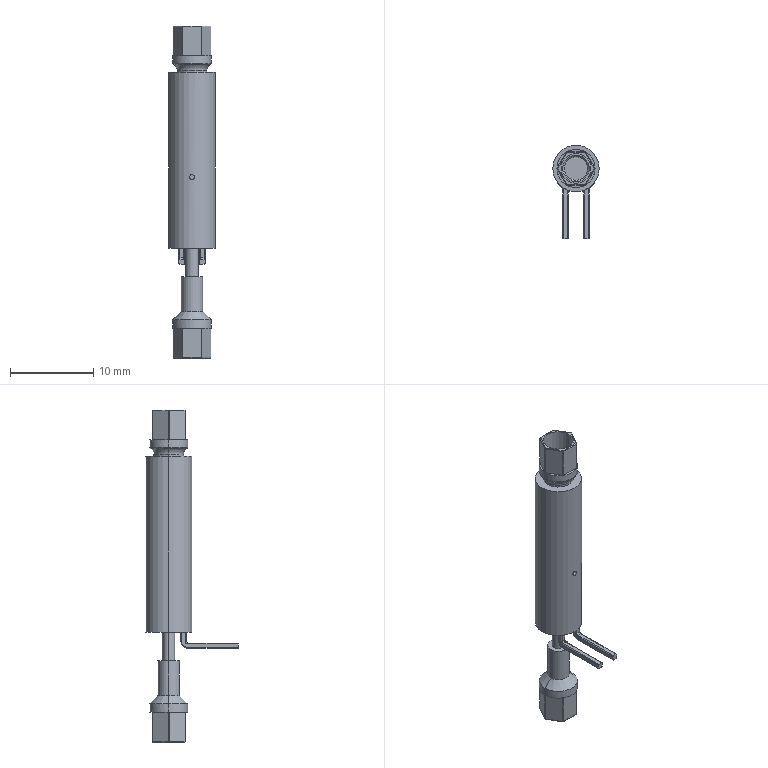Part | SolidWorks | features Boss 6, Cut 3, Fillet 3, MirrorPattern 3, Chamfer 1, Extrusion 1, Sweep 1 | 1 solid | 133 faces | box 5.6 x 11.2 x 40 mm | volume 624.39 mm3 | cylinder 66 | plane 37 | sphere 14 | torus 12 | cone 4 | commonest cylinder face diameters 0.16 x26 0.2 x16 3.6 x6 4.6 x4 0.36 x2 0.6 x2